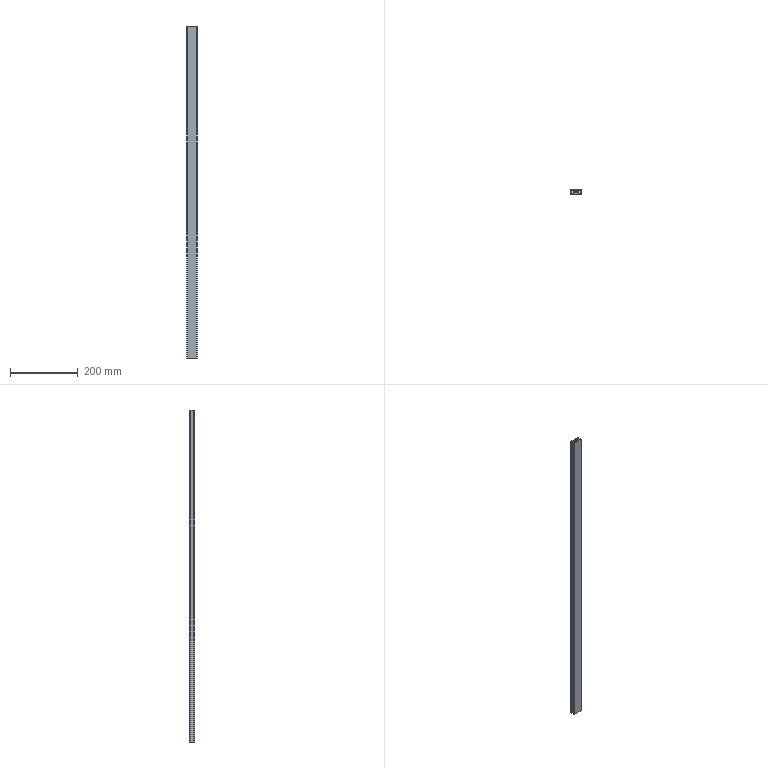Part | SolidWorks | features BaseBody 1, MoveFace 1 | 1 solid | 53 faces | box 30 x 15 x 983 mm | volume 237069 mm3 | plane 38 | cylinder 15 | commonest cylinder face diameters 1 x6 5 x5 2 x4